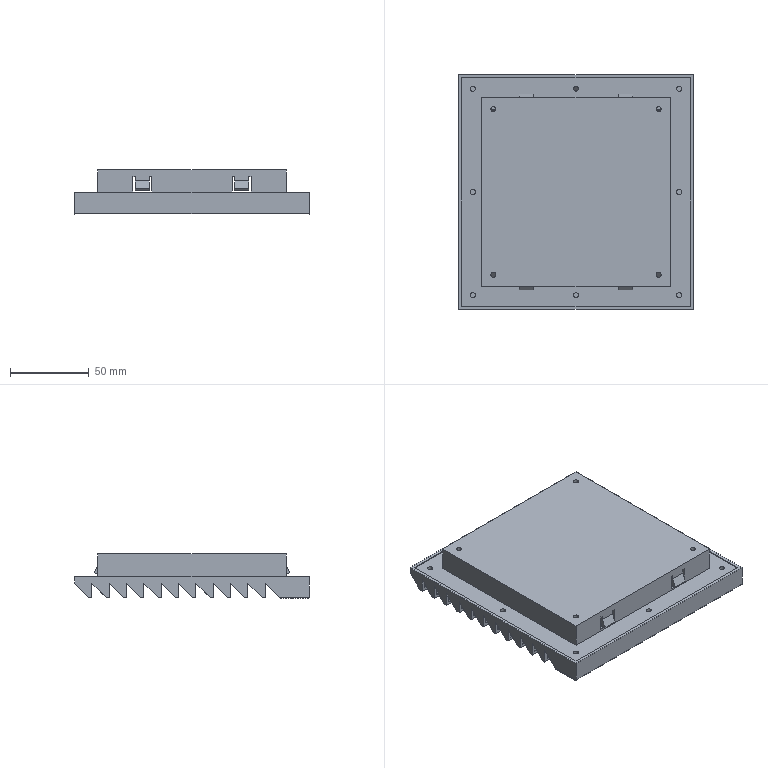Part | STEP file | Ventilation filter assembly-KM | 1 solid | 351 faces | box 149 x 149 x 28 mm | volume 126448 mm3 | plane 315 | cylinder 36 | commonest cylinder face diameters 3.242 x24 1 x12